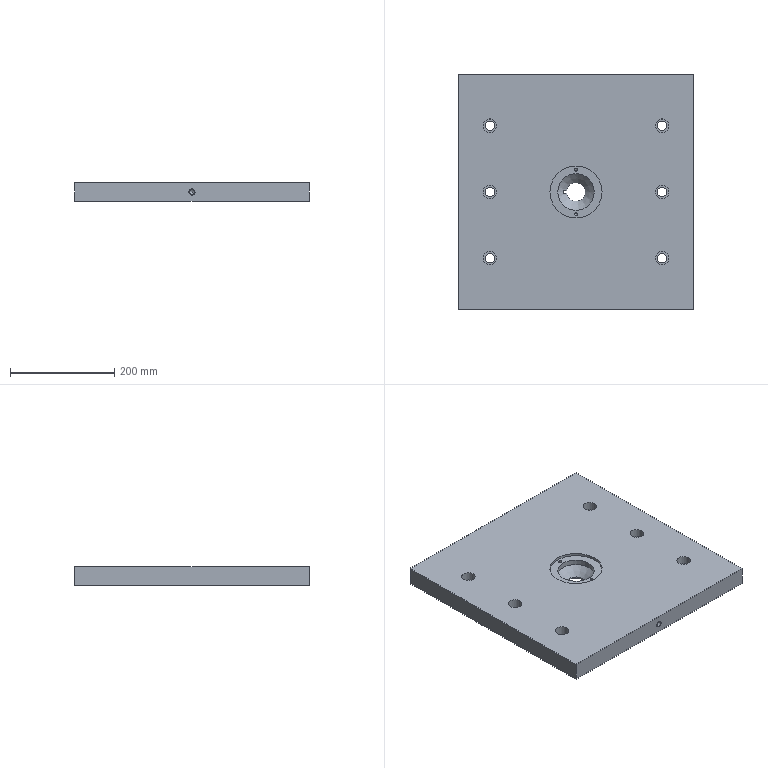Part | NX | features solid 2 | 1 solid | 71 faces | box 450 x 450 x 35 mm | volume 6878672 mm3 | plane 38 | cylinder 28 | cone 5 | commonest cylinder face diameters 18 x6 26 x6 5 x3 5.7 x2 6 x2 10.2 x2